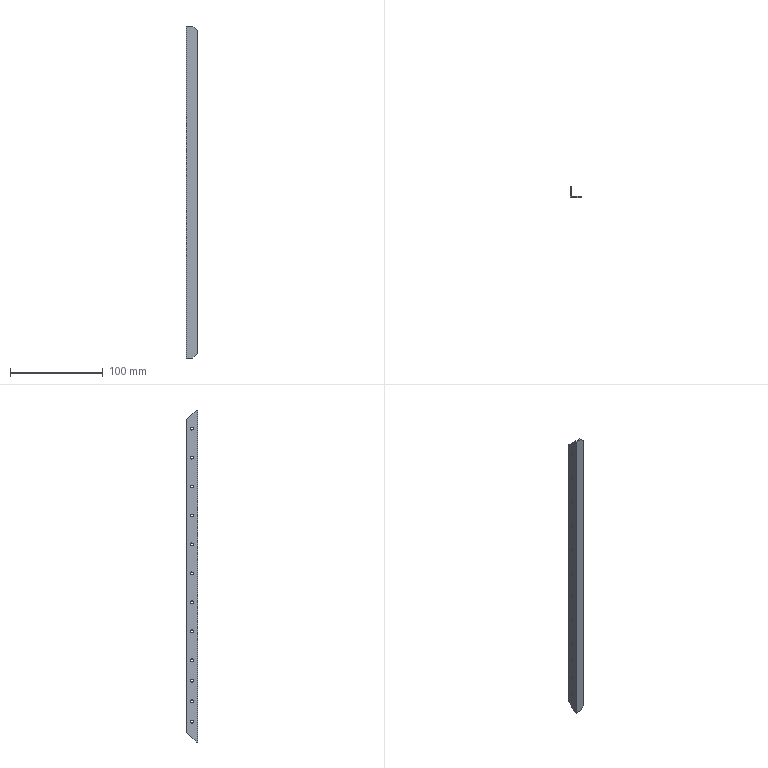Part | SolidWorks | features BaseBody 1 | 1 solid | 36 faces | box 12 x 12 x 358 mm | volume 9517 mm3 | cylinder 24 | plane 12 | commonest cylinder face diameters 3.2 x24
STEP:
#1=CARTESIAN_POINT('',(1.2,6.015,129.35));
#2=VERTEX_POINT('',#1);
#3=CARTESIAN_POINT('',(1.2,6.015,126.15));
#4=VERTEX_POINT('',#3);
#5=CARTESIAN_POINT('',(1.2,6.015,127.75));
#6=DIRECTION('',(1.,0.,0.));
#7=DIRECTION('',(0.,0.,1.));
#8=AXIS2_PLACEMENT_3D('',#5,#6,#7);
#9=CIRCLE('',#8,1.6);
#10=EDGE_CURVE('',#2,#4,#9,.T.);
#11=ORIENTED_EDGE('',*,*,#10,.T.);
#12=CARTESIAN_POINT('',(0.,6.015,126.15));
#13=VERTEX_POINT('',#12);
#14=CARTESIAN_POINT('',(1.2,6.015,126.15));
#15=DIRECTION('',(-1.,0.,0.));
#16=VECTOR('',#15,1000.);
#17=LINE('',#14,#16);
#18=EDGE_CURVE('',#4,#13,#17,.T.);
#19=ORIENTED_EDGE('',*,*,#18,.T.);
#20=CARTESIAN_POINT('',(0.,6.015,129.35));
#21=VERTEX_POINT('',#20);
#22=CARTESIAN_POINT('',(0.,6.015,127.75));
#23=DIRECTION('',(-1.,0.,0.));
#24=DIRECTION('',(0.,0.,1.));
#25=AXIS2_PLACEMENT_3D('',#22,#23,#24);
#26=CIRCLE('',#25,1.6);
#27=EDGE_CURVE('',#13,#21,#26,.T.);
#28=ORIENTED_EDGE('',*,*,#27,.T.);
#29=CARTESIAN_POINT('',(1.2,6.015,129.35));
#30=DIRECTION('',(-1.,0.,0.));
#31=VECTOR('',#30,1000.);
#32=LINE('',#29,#31);
#33=EDGE_CURVE('',#2,#21,#32,.T.);
#34=ORIENTED_EDGE('',*,*,#33,.F.);
#35=EDGE_LOOP('',(#11,#19,#28,#34));
#36=FACE_OUTER_BOUND('',#35,.T.);
#37=CARTESIAN_POINT('',(1.2,6.015,127.75));
#38=DIRECTION('',(-1.,0.,0.));
#39=DIRECTION('',(0.,0.,1.));
#40=AXIS2_PLACEMENT_3D('',#37,#38,#39);
#41=CYLINDRICAL_SURFACE('',#40,1.6);
#42=ADVANCED_FACE('',(#36),#41,.F.);
#43=CARTESIAN_POINT('',(1.2,6.015,-155.4));
#44=VERTEX_POINT('',#43);
#45=CARTESIAN_POINT('',(1.2,6.015,-158.6));
#46=VERTEX_POINT('',#45);
#47=CARTESIAN_POINT('',(1.2,6.015,-157.));
#48=DIRECTION('',(1.,0.,0.));
#49=DIRECTION('',(0.,0.,1.));
#50=AXIS2_PLACEMENT_3D('',#47,#48,#49);
#51=CIRCLE('',#50,1.6);
#52=EDGE_CURVE('',#44,#46,#51,.T.);
#53=ORIENTED_EDGE('',*,*,#52,.T.);
#54=CARTESIAN_POINT('',(0.,6.015,-158.6));
#55=VERTEX_POINT('',#54);
#56=CARTESIAN_POINT('',(1.2,6.015,-158.6));
#57=DIRECTION('',(-1.,0.,0.));
#58=VECTOR('',#57,1000.);
#59=LINE('',#56,#58);
#60=EDGE_CURVE('',#46,#55,#59,.T.);
#61=ORIENTED_EDGE('',*,*,#60,.T.);
#62=CARTESIAN_POINT('',(0.,6.015,-155.4));
#63=VERTEX_POINT('',#62);
#64=CARTESIAN_POINT('',(0.,6.015,-157.));
#65=DIRECTION('',(-1.,0.,0.));
#66=DIRECTION('',(0.,0.,1.));
#67=AXIS2_PLACEMENT_3D('',#64,#65,#66);
#68=CIRCLE('',#67,1.6);
#69=EDGE_CURVE('',#55,#63,#68,.T.);
#70=ORIENTED_EDGE('',*,*,#69,.T.);
#71=CARTESIAN_POINT('',(1.2,6.015,-155.4));
#72=DIRECTION('',(-1.,0.,0.));
#73=VECTOR('',#72,1000.);
#74=LINE('',#71,#73);
#75=EDGE_CURVE('',#44,#63,#74,.T.);
#76=ORIENTED_EDGE('',*,*,#75,.F.);
#77=EDGE_LOOP('',(#53,#61,#70,#76));
#78=FACE_OUTER_BOUND('',#77,.T.);
#79=CARTESIAN_POINT('',(1.2,6.015,-157.));
#80=DIRECTION('',(-1.,0.,0.));
#81=DIRECTION('',(0.,0.,1.));
#82=AXIS2_PLACEMENT_3D('',#79,#80,#81);
#83=CYLINDRICAL_SURFACE('',#82,1.6);
#84=ADVANCED_FACE('',(#78),#83,.F.);
#85=CARTESIAN_POINT('',(1.2,6.015,160.6));
#86=VERTEX_POINT('',#85);
#87=CARTESIAN_POINT('',(1.2,6.015,157.4));
#88=VERTEX_POINT('',#87);
#89=CARTESIAN_POINT('',(1.2,6.015,159.));
#90=DIRECTION('',(1.,0.,0.));
#91=DIRECTION('',(0.,0.,1.));
#92=AXIS2_PLACEMENT_3D('',#89,#90,#91);
#93=CIRCLE('',#92,1.6);
#94=EDGE_CURVE('',#86,#88,#93,.T.);
#95=ORIENTED_EDGE('',*,*,#94,.T.);
#96=CARTESIAN_POINT('',(0.,6.015,157.4));
#97=VERTEX_POINT('',#96);
#98=CARTESIAN_POINT('',(1.2,6.015,157.4));
#99=DIRECTION('',(-1.,0.,0.));
#100=VECTOR('',#99,1000.);
#101=LINE('',#98,#100);
#102=EDGE_CURVE('',#88,#97,#101,.T.);
#103=ORIENTED_EDGE('',*,*,#102,.T.);
#104=CARTESIAN_POINT('',(0.,6.015,160.6));
#105=VERTEX_POINT('',#104);
#106=CARTESIAN_POINT('',(0.,6.015,159.));
#107=DIRECTION('',(-1.,0.,0.));
#108=DIRECTION('',(0.,0.,1.));
#109=AXIS2_PLACEMENT_3D('',#106,#107,#108);
#110=CIRCLE('',#109,1.6);
#111=EDGE_CURVE('',#97,#105,#110,.T.);
#112=ORIENTED_EDGE('',*,*,#111,.T.);
#113=CARTESIAN_POINT('',(1.2,6.015,160.6));
#114=DIRECTION('',(-1.,0.,0.));
#115=VECTOR('',#114,1000.);
#116=LINE('',#113,#115);
#117=EDGE_CURVE('',#86,#105,#116,.T.);
#118=ORIENTED_EDGE('',*,*,#117,.F.);
#119=EDGE_LOOP('',(#95,#103,#112,#118));
#120=FACE_OUTER_BOUND('',#119,.T.);
#121=CARTESIAN_POINT('',(1.2,6.015,159.));
#122=DIRECTION('',(-1.,0.,0.));
#123=DIRECTION('',(0.,0.,1.));
#124=AXIS2_PLACEMENT_3D('',#121,#122,#123);
#125=CYLINDRICAL_SURFACE('',#124,1.6);
#126=ADVANCED_FACE('',(#120),#125,.F.);
#127=CARTESIAN_POINT('',(1.2,6.015,-133.4));
#128=VERTEX_POINT('',#127);
#129=CARTESIAN_POINT('',(1.2,6.015,-136.6));
#130=VERTEX_POINT('',#129);
#131=CARTESIAN_POINT('',(1.2,6.015,-135.));
#132=DIRECTION('',(1.,0.,0.));
#133=DIRECTION('',(0.,0.,1.));
#134=AXIS2_PLACEMENT_3D('',#131,#132,#133);
#135=CIRCLE('',#134,1.6);
#136=EDGE_CURVE('',#128,#130,#135,.T.);
#137=ORIENTED_EDGE('',*,*,#136,.T.);
#138=CARTESIAN_POINT('',(0.,6.015,-136.6));
#139=VERTEX_POINT('',#138);
#140=CARTESIAN_POINT('',(1.2,6.015,-136.6));
#141=DIRECTION('',(-1.,0.,0.));
#142=VECTOR('',#141,1000.);
#143=LINE('',#140,#142);
#144=EDGE_CURVE('',#130,#139,#143,.T.);
#145=ORIENTED_EDGE('',*,*,#144,.T.);
#146=CARTESIAN_POINT('',(0.,6.015,-133.4));
#147=VERTEX_POINT('',#146);
#148=CARTESIAN_POINT('',(0.,6.015,-135.));
#149=DIRECTION('',(-1.,0.,0.));
#150=DIRECTION('',(0.,0.,1.));
#151=AXIS2_PLACEMENT_3D('',#148,#149,#150);
#152=CIRCLE('',#151,1.6);
#153=EDGE_CURVE('',#139,#147,#152,.T.);
#154=ORIENTED_EDGE('',*,*,#153,.T.);
#155=CARTESIAN_POINT('',(1.2,6.015,-133.4));
#156=DIRECTION('',(-1.,0.,0.));
#157=VECTOR('',#156,1000.);
#158=LINE('',#155,#157);
#159=EDGE_CURVE('',#128,#147,#158,.T.);
#160=ORIENTED_EDGE('',*,*,#159,.F.);
#161=EDGE_LOOP('',(#137,#145,#154,#160));
#162=FACE_OUTER_BOUND('',#161,.T.);
#163=CARTESIAN_POINT('',(1.2,6.015,-135.));
#164=DIRECTION('',(-1.,0.,0.));
#165=DIRECTION('',(0.,0.,1.));
#166=AXIS2_PLACEMENT_3D('',#163,#164,#165);
#167=CYLINDRICAL_SURFACE('',#166,1.6);
#168=ADVANCED_FACE('',(#162),#167,.F.);
#169=CARTESIAN_POINT('',(1.2,6.015,-111.4));
#170=VERTEX_POINT('',#169);
#171=CARTESIAN_POINT('',(1.2,6.015,-114.6));
#172=VERTEX_POINT('',#171);
#173=CARTESIAN_POINT('',(1.2,6.015,-113.));
#174=DIRECTION('',(1.,0.,0.));
#175=DIRECTION('',(0.,0.,1.));
#176=AXIS2_PLACEMENT_3D('',#173,#174,#175);
#177=CIRCLE('',#176,1.6);
#178=EDGE_CURVE('',#170,#172,#177,.T.);
#179=ORIENTED_EDGE('',*,*,#178,.T.);
#180=CARTESIAN_POINT('',(0.,6.015,-114.6));
#181=VERTEX_POINT('',#180);
#182=CARTESIAN_POINT('',(1.2,6.015,-114.6));
#183=DIRECTION('',(-1.,0.,0.));
#184=VECTOR('',#183,1000.);
#185=LINE('',#182,#184);
#186=EDGE_CURVE('',#172,#181,#185,.T.);
#187=ORIENTED_EDGE('',*,*,#186,.T.);
#188=CARTESIAN_POINT('',(0.,6.015,-111.4));
#189=VERTEX_POINT('',#188);
#190=CARTESIAN_POINT('',(0.,6.015,-113.));
#191=DIRECTION('',(-1.,0.,0.));
#192=DIRECTION('',(0.,0.,1.));
#193=AXIS2_PLACEMENT_3D('',#190,#191,#192);
#194=CIRCLE('',#193,1.6);
#195=EDGE_CURVE('',#181,#189,#194,.T.);
#196=ORIENTED_EDGE('',*,*,#195,.T.);
#197=CARTESIAN_POINT('',(1.2,6.015,-111.4));
#198=DIRECTION('',(-1.,0.,0.));
#199=VECTOR('',#198,1000.);
#200=LINE('',#197,#199);
#201=EDGE_CURVE('',#170,#189,#200,.T.);
#202=ORIENTED_EDGE('',*,*,#201,.F.);
#203=EDGE_LOOP('',(#179,#187,#196,#202));
#204=FACE_OUTER_BOUND('',#203,.T.);
#205=CARTESIAN_POINT('',(1.2,6.015,-113.));
#206=DIRECTION('',(-1.,0.,0.));
#207=DIRECTION('',(0.,0.,1.));
#208=AXIS2_PLACEMENT_3D('',#205,#206,#207);
#209=CYLINDRICAL_SURFACE('',#208,1.6);
#210=ADVANCED_FACE('',(#204),#209,.F.);
#211=CARTESIAN_POINT('',(1.2,6.015,-89.4));
#212=VERTEX_POINT('',#211);
#213=CARTESIAN_POINT('',(1.2,6.015,-92.6));
#214=VERTEX_POINT('',#213);
#215=CARTESIAN_POINT('',(1.2,6.015,-91.));
#216=DIRECTION('',(1.,0.,0.));
#217=DIRECTION('',(0.,0.,1.));
#218=AXIS2_PLACEMENT_3D('',#215,#216,#217);
#219=CIRCLE('',#218,1.6);
#220=EDGE_CURVE('',#212,#214,#219,.T.);
#221=ORIENTED_EDGE('',*,*,#220,.T.);
#222=CARTESIAN_POINT('',(0.,6.015,-92.6));
#223=VERTEX_POINT('',#222);
#224=CARTESIAN_POINT('',(1.2,6.015,-92.6));
#225=DIRECTION('',(-1.,0.,0.));
#226=VECTOR('',#225,1000.);
#227=LINE('',#224,#226);
#228=EDGE_CURVE('',#214,#223,#227,.T.);
#229=ORIENTED_EDGE('',*,*,#228,.T.);
#230=CARTESIAN_POINT('',(0.,6.015,-89.4));
#231=VERTEX_POINT('',#230);
#232=CARTESIAN_POINT('',(0.,6.015,-91.));
#233=DIRECTION('',(-1.,0.,0.));
#234=DIRECTION('',(0.,0.,1.));
#235=AXIS2_PLACEMENT_3D('',#232,#233,#234);
#236=CIRCLE('',#235,1.6);
#237=EDGE_CURVE('',#223,#231,#236,.T.);
#238=ORIENTED_EDGE('',*,*,#237,.T.);
#239=CARTESIAN_POINT('',(1.2,6.015,-89.4));
#240=DIRECTION('',(-1.,0.,0.));
#241=VECTOR('',#240,1000.);
#242=LINE('',#239,#241);
#243=EDGE_CURVE('',#212,#231,#242,.T.);
#244=ORIENTED_EDGE('',*,*,#243,.F.);
#245=EDGE_LOOP('',(#221,#229,#238,#244));
#246=FACE_OUTER_BOUND('',#245,.T.);
#247=CARTESIAN_POINT('',(1.2,6.015,-91.));
#248=DIRECTION('',(-1.,0.,0.));
#249=DIRECTION('',(0.,0.,1.));
#250=AXIS2_PLACEMENT_3D('',#247,#248,#249);
#251=CYLINDRICAL_SURFACE('',#250,1.6);
#252=ADVANCED_FACE('',(#246),#251,.F.);
#253=CARTESIAN_POINT('',(1.2,6.015,-58.15));
#254=VERTEX_POINT('',#253);
#255=CARTESIAN_POINT('',(1.2,6.015,-61.35));
#256=VERTEX_POINT('',#255);
#257=CARTESIAN_POINT('',(1.2,6.015,-59.75));
#258=DIRECTION('',(1.,0.,0.));
#259=DIRECTION('',(0.,0.,1.));
#260=AXIS2_PLACEMENT_3D('',#257,#258,#259);
#261=CIRCLE('',#260,1.6);
#262=EDGE_CURVE('',#254,#256,#261,.T.);
#263=ORIENTED_EDGE('',*,*,#262,.T.);
#264=CARTESIAN_POINT('',(0.,6.015,-61.35));
#265=VERTEX_POINT('',#264);
#266=CARTESIAN_POINT('',(1.2,6.015,-61.35));
#267=DIRECTION('',(-1.,0.,0.));
#268=VECTOR('',#267,1000.);
#269=LINE('',#266,#268);
#270=EDGE_CURVE('',#256,#265,#269,.T.);
#271=ORIENTED_EDGE('',*,*,#270,.T.);
#272=CARTESIAN_POINT('',(0.,6.015,-58.15));
#273=VERTEX_POINT('',#272);
#274=CARTESIAN_POINT('',(0.,6.015,-59.75));
#275=DIRECTION('',(-1.,0.,0.));
#276=DIRECTION('',(0.,0.,1.));
#277=AXIS2_PLACEMENT_3D('',#274,#275,#276);
#278=CIRCLE('',#277,1.6);
#279=EDGE_CURVE('',#265,#273,#278,.T.);
#280=ORIENTED_EDGE('',*,*,#279,.T.);
#281=CARTESIAN_POINT('',(1.2,6.015,-58.15));
#282=DIRECTION('',(-1.,0.,0.));
#283=VECTOR('',#282,1000.);
#284=LINE('',#281,#283);
#285=EDGE_CURVE('',#254,#273,#284,.T.);
#286=ORIENTED_EDGE('',*,*,#285,.F.);
#287=EDGE_LOOP('',(#263,#271,#280,#286));
#288=FACE_OUTER_BOUND('',#287,.T.);
#289=CARTESIAN_POINT('',(1.2,6.015,-59.75));
#290=DIRECTION('',(-1.,0.,0.));
#291=DIRECTION('',(0.,0.,1.));
#292=AXIS2_PLACEMENT_3D('',#289,#290,#291);
#293=CYLINDRICAL_SURFACE('',#292,1.6);
#294=ADVANCED_FACE('',(#288),#293,.F.);
#295=CARTESIAN_POINT('',(1.2,6.015,-26.9));
#296=VERTEX_POINT('',#295);
#297=CARTESIAN_POINT('',(1.2,6.015,-30.1));
#298=VERTEX_POINT('',#297);
#299=CARTESIAN_POINT('',(1.2,6.015,-28.5));
#300=DIRECTION('',(1.,0.,0.));
#301=DIRECTION('',(0.,0.,1.));
#302=AXIS2_PLACEMENT_3D('',#299,#300,#301);
#303=CIRCLE('',#302,1.6);
#304=EDGE_CURVE('',#296,#298,#303,.T.);
#305=ORIENTED_EDGE('',*,*,#304,.T.);
#306=CARTESIAN_POINT('',(0.,6.015,-30.1));
#307=VERTEX_POINT('',#306);
#308=CARTESIAN_POINT('',(1.2,6.015,-30.1));
#309=DIRECTION('',(-1.,0.,0.));
#310=VECTOR('',#309,1000.);
#311=LINE('',#308,#310);
#312=EDGE_CURVE('',#298,#307,#311,.T.);
#313=ORIENTED_EDGE('',*,*,#312,.T.);
#314=CARTESIAN_POINT('',(0.,6.015,-26.9));
#315=VERTEX_POINT('',#314);
#316=CARTESIAN_POINT('',(0.,6.015,-28.5));
#317=DIRECTION('',(-1.,0.,0.));
#318=DIRECTION('',(0.,0.,1.));
#319=AXIS2_PLACEMENT_3D('',#316,#317,#318);
#320=CIRCLE('',#319,1.6);
#321=EDGE_CURVE('',#307,#315,#320,.T.);
#322=ORIENTED_EDGE('',*,*,#321,.T.);
#323=CARTESIAN_POINT('',(1.2,6.015,-26.9));
#324=DIRECTION('',(-1.,0.,0.));
#325=VECTOR('',#324,1000.);
#326=LINE('',#323,#325);
#327=EDGE_CURVE('',#296,#315,#326,.T.);
#328=ORIENTED_EDGE('',*,*,#327,.F.);
#329=EDGE_LOOP('',(#305,#313,#322,#328));
#330=FACE_OUTER_BOUND('',#329,.T.);
#331=CARTESIAN_POINT('',(1.2,6.015,-28.5));
#332=DIRECTION('',(-1.,0.,0.));
#333=DIRECTION('',(0.,0.,1.));
#334=AXIS2_PLACEMENT_3D('',#331,#332,#333);
#335=CYLINDRICAL_SURFACE('',#334,1.6);
#336=ADVANCED_FACE('',(#330),#335,.F.);
#337=CARTESIAN_POINT('',(1.2,6.015,4.35));
#338=VERTEX_POINT('',#337);
#339=CARTESIAN_POINT('',(1.2,6.015,1.15));
#340=VERTEX_POINT('',#339);
#341=CARTESIAN_POINT('',(1.2,6.015,2.75));
#342=DIRECTION('',(1.,0.,0.));
#343=DIRECTION('',(0.,0.,1.));
#344=AXIS2_PLACEMENT_3D('',#341,#342,#343);
#345=CIRCLE('',#344,1.6);
#346=EDGE_CURVE('',#338,#340,#345,.T.);
#347=ORIENTED_EDGE('',*,*,#346,.T.);
#348=CARTESIAN_POINT('',(0.,6.015,1.15));
#349=VERTEX_POINT('',#348);
#350=CARTESIAN_POINT('',(1.2,6.015,1.15));
#351=DIRECTION('',(-1.,0.,0.));
#352=VECTOR('',#351,1000.);
#353=LINE('',#350,#352);
#354=EDGE_CURVE('',#340,#349,#353,.T.);
#355=ORIENTED_EDGE('',*,*,#354,.T.);
#356=CARTESIAN_POINT('',(0.,6.015,4.35));
#357=VERTEX_POINT('',#356);
#358=CARTESIAN_POINT('',(0.,6.015,2.75));
#359=DIRECTION('',(-1.,0.,0.));
#360=DIRECTION('',(0.,0.,1.));
#361=AXIS2_PLACEMENT_3D('',#358,#359,#360);
#362=CIRCLE('',#361,1.6);
#363=EDGE_CURVE('',#349,#357,#362,.T.);
#364=ORIENTED_EDGE('',*,*,#363,.T.);
#365=CARTESIAN_POINT('',(1.2,6.015,4.35));
#366=DIRECTION('',(-1.,0.,0.));
#367=VECTOR('',#366,1000.);
#368=LINE('',#365,#367);
#369=EDGE_CURVE('',#338,#357,#368,.T.);
#370=ORIENTED_EDGE('',*,*,#369,.F.);
#371=EDGE_LOOP('',(#347,#355,#364,#370));
#372=FACE_OUTER_BOUND('',#371,.T.);
#373=CARTESIAN_POINT('',(1.2,6.015,2.75));
#374=DIRECTION('',(-1.,0.,0.));
#375=DIRECTION('',(0.,0.,1.));
#376=AXIS2_PLACEMENT_3D('',#373,#374,#375);
#377=CYLINDRICAL_SURFACE('',#376,1.6);
#378=ADVANCED_FACE('',(#372),#377,.F.);
#379=CARTESIAN_POINT('',(1.2,6.015,35.6));
#380=VERTEX_POINT('',#379);
#381=CARTESIAN_POINT('',(1.2,6.015,32.4));
#382=VERTEX_POINT('',#381);
#383=CARTESIAN_POINT('',(1.2,6.015,34.));
#384=DIRECTION('',(1.,0.,0.));
#385=DIRECTION('',(0.,0.,1.));
#386=AXIS2_PLACEMENT_3D('',#383,#384,#385);
#387=CIRCLE('',#386,1.6);
#388=EDGE_CURVE('',#380,#382,#387,.T.);
#389=ORIENTED_EDGE('',*,*,#388,.T.);
#390=CARTESIAN_POINT('',(0.,6.015,32.4));
#391=VERTEX_POINT('',#390);
#392=CARTESIAN_POINT('',(1.2,6.015,32.4));
#393=DIRECTION('',(-1.,0.,0.));
#394=VECTOR('',#393,1000.);
#395=LINE('',#392,#394);
#396=EDGE_CURVE('',#382,#391,#395,.T.);
#397=ORIENTED_EDGE('',*,*,#396,.T.);
#398=CARTESIAN_POINT('',(0.,6.015,35.6));
#399=VERTEX_POINT('',#398);
#400=CARTESIAN_POINT('',(0.,6.015,34.));
#401=DIRECTION('',(-1.,0.,0.));
#402=DIRECTION('',(0.,0.,1.));
#403=AXIS2_PLACEMENT_3D('',#400,#401,#402);
#404=CIRCLE('',#403,1.6);
#405=EDGE_CURVE('',#391,#399,#404,.T.);
#406=ORIENTED_EDGE('',*,*,#405,.T.);
#407=CARTESIAN_POINT('',(1.2,6.015,35.6));
#408=DIRECTION('',(-1.,0.,0.));
#409=VECTOR('',#408,1000.);
#410=LINE('',#407,#409);
#411=EDGE_CURVE('',#380,#399,#410,.T.);
#412=ORIENTED_EDGE('',*,*,#411,.F.);
#413=EDGE_LOOP('',(#389,#397,#406,#412));
#414=FACE_OUTER_BOUND('',#413,.T.);
#415=CARTESIAN_POINT('',(1.2,6.015,34.));
#416=DIRECTION('',(-1.,0.,0.));
#417=DIRECTION('',(0.,0.,1.));
#418=AXIS2_PLACEMENT_3D('',#415,#416,#417);
#419=CYLINDRICAL_SURFACE('',#418,1.6);
#420=ADVANCED_FACE('',(#414),#419,.F.);
#421=CARTESIAN_POINT('',(1.2,6.015,66.85));
#422=VERTEX_POINT('',#421);
#423=CARTESIAN_POINT('',(1.2,6.015,63.65));
#424=VERTEX_POINT('',#423);
#425=CARTESIAN_POINT('',(1.2,6.015,65.25));
#426=DIRECTION('',(1.,0.,0.));
#427=DIRECTION('',(0.,0.,1.));
#428=AXIS2_PLACEMENT_3D('',#425,#426,#427);
#429=CIRCLE('',#428,1.6);
#430=EDGE_CURVE('',#422,#424,#429,.T.);
#431=ORIENTED_EDGE('',*,*,#430,.T.);
#432=CARTESIAN_POINT('',(0.,6.015,63.65));
#433=VERTEX_POINT('',#432);
#434=CARTESIAN_POINT('',(1.2,6.015,63.65));
#435=DIRECTION('',(-1.,0.,0.));
#436=VECTOR('',#435,1000.);
#437=LINE('',#434,#436);
#438=EDGE_CURVE('',#424,#433,#437,.T.);
#439=ORIENTED_EDGE('',*,*,#438,.T.);
#440=CARTESIAN_POINT('',(0.,6.015,66.85));
#441=VERTEX_POINT('',#440);
#442=CARTESIAN_POINT('',(0.,6.015,65.25));
#443=DIRECTION('',(-1.,0.,0.));
#444=DIRECTION('',(0.,0.,1.));
#445=AXIS2_PLACEMENT_3D('',#442,#443,#444);
#446=CIRCLE('',#445,1.6);
#447=EDGE_CURVE('',#433,#441,#446,.T.);
#448=ORIENTED_EDGE('',*,*,#447,.T.);
#449=CARTESIAN_POINT('',(1.2,6.015,66.85));
#450=DIRECTION('',(-1.,0.,0.));
#451=VECTOR('',#450,1000.);
#452=LINE('',#449,#451);
#453=EDGE_CURVE('',#422,#441,#452,.T.);
#454=ORIENTED_EDGE('',*,*,#453,.F.);
#455=EDGE_LOOP('',(#431,#439,#448,#454));
#456=FACE_OUTER_BOUND('',#455,.T.);
#457=CARTESIAN_POINT('',(1.2,6.015,65.25));
#458=DIRECTION('',(-1.,0.,0.));
#459=DIRECTION('',(0.,0.,1.));
#460=AXIS2_PLACEMENT_3D('',#457,#458,#459);
#461=CYLINDRICAL_SURFACE('',#460,1.6);
#462=ADVANCED_FACE('',(#456),#461,.F.);
#463=CARTESIAN_POINT('',(1.2,6.015,98.1));
#464=VERTEX_POINT('',#463);
#465=CARTESIAN_POINT('',(1.2,6.015,94.9));
#466=VERTEX_POINT('',#465);
#467=CARTESIAN_POINT('',(1.2,6.015,96.5));
#468=DIRECTION('',(1.,0.,0.));
#469=DIRECTION('',(0.,0.,1.));
#470=AXIS2_PLACEMENT_3D('',#467,#468,#469);
#471=CIRCLE('',#470,1.6);
#472=EDGE_CURVE('',#464,#466,#471,.T.);
#473=ORIENTED_EDGE('',*,*,#472,.T.);
#474=CARTESIAN_POINT('',(0.,6.015,94.9));
#475=VERTEX_POINT('',#474);
#476=CARTESIAN_POINT('',(1.2,6.015,94.9));
#477=DIRECTION('',(-1.,0.,0.));
#478=VECTOR('',#477,1000.);
#479=LINE('',#476,#478);
#480=EDGE_CURVE('',#466,#475,#479,.T.);
#481=ORIENTED_EDGE('',*,*,#480,.T.);
#482=CARTESIAN_POINT('',(0.,6.015,98.1));
#483=VERTEX_POINT('',#482);
#484=CARTESIAN_POINT('',(0.,6.015,96.5));
#485=DIRECTION('',(-1.,0.,0.));
#486=DIRECTION('',(0.,0.,1.));
#487=AXIS2_PLACEMENT_3D('',#484,#485,#486);
#488=CIRCLE('',#487,1.6);
#489=EDGE_CURVE('',#475,#483,#488,.T.);
#490=ORIENTED_EDGE('',*,*,#489,.T.);
#491=CARTESIAN_POINT('',(1.2,6.015,98.1));
#492=DIRECTION('',(-1.,0.,0.));
#493=VECTOR('',#492,1000.);
#494=LINE('',#491,#493);
#495=EDGE_CURVE('',#464,#483,#494,.T.);
#496=ORIENTED_EDGE('',*,*,#495,.F.);
#497=EDGE_LOOP('',(#473,#481,#490,#496));
#498=FACE_OUTER_BOUND('',#497,.T.);
#499=CARTESIAN_POINT('',(1.2,6.015,96.5));
#500=DIRECTION('',(-1.,0.,0.));
#501=DIRECTION('',(0.,0.,1.));
#502=AXIS2_PLACEMENT_3D('',#499,#500,#501);
#503=CYLINDRICAL_SURFACE('',#502,1.6);
#504=ADVANCED_FACE('',(#498),#503,.F.);
#505=ORIENTED_EDGE('',*,*,#18,.F.);
#506=CARTESIAN_POINT('',(1.2,6.015,127.75));
#507=DIRECTION('',(1.,0.,0.));
#508=DIRECTION('',(0.,0.,1.));
#509=AXIS2_PLACEMENT_3D('',#506,#507,#508);
#510=CIRCLE('',#509,1.6);
#511=EDGE_CURVE('',#4,#2,#510,.T.);
#512=ORIENTED_EDGE('',*,*,#511,.T.);
#513=ORIENTED_EDGE('',*,*,#33,.T.);
#514=CARTESIAN_POINT('',(0.,6.015,127.75));
#515=DIRECTION('',(-1.,0.,0.));
#516=DIRECTION('',(0.,0.,1.));
#517=AXIS2_PLACEMENT_3D('',#514,#515,#516);
#518=CIRCLE('',#517,1.6);
#519=EDGE_CURVE('',#21,#13,#518,.T.);
#520=ORIENTED_EDGE('',*,*,#519,.T.);
#521=EDGE_LOOP('',(#505,#512,#513,#520));
#522=FACE_OUTER_BOUND('',#521,.T.);
#523=CARTESIAN_POINT('',(1.2,6.015,127.75));
#524=DIRECTION('',(-1.,0.,0.));
#525=DIRECTION('',(0.,0.,1.));
#526=AXIS2_PLACEMENT_3D('',#523,#524,#525);
#527=CYLINDRICAL_SURFACE('',#526,1.6);
#528=ADVANCED_FACE('',(#522),#527,.F.);
#529=CARTESIAN_POINT('',(0.,6.015,-157.));
#530=DIRECTION('',(-1.,0.,0.));
#531=DIRECTION('',(0.,0.,1.));
#532=AXIS2_PLACEMENT_3D('',#529,#530,#531);
#533=CIRCLE('',#532,1.6);
#534=EDGE_CURVE('',#63,#55,#533,.T.);
#535=ORIENTED_EDGE('',*,*,#534,.F.);
#536=ORIENTED_EDGE('',*,*,#69,.F.);
#537=EDGE_LOOP('',(#535,#536));
#538=FACE_BOUND('',#537,.T.);
#539=CARTESIAN_POINT('',(0.,6.015,159.));
#540=DIRECTION('',(-1.,0.,0.));
#541=DIRECTION('',(0.,0.,1.));
#542=AXIS2_PLACEMENT_3D('',#539,#540,#541);
#543=CIRCLE('',#542,1.6);
#544=EDGE_CURVE('',#105,#97,#543,.T.);
#545=ORIENTED_EDGE('',*,*,#544,.F.);
#546=ORIENTED_EDGE('',*,*,#111,.F.);
#547=EDGE_LOOP('',(#545,#546));
#548=FACE_BOUND('',#547,.T.);
#549=CARTESIAN_POINT('',(0.,6.015,-135.));
#550=DIRECTION('',(-1.,0.,0.));
#551=DIRECTION('',(0.,0.,1.));
#552=AXIS2_PLACEMENT_3D('',#549,#550,#551);
#553=CIRCLE('',#552,1.6);
#554=EDGE_CURVE('',#147,#139,#553,.T.);
#555=ORIENTED_EDGE('',*,*,#554,.F.);
#556=ORIENTED_EDGE('',*,*,#153,.F.);
#557=EDGE_LOOP('',(#555,#556));
#558=FACE_BOUND('',#557,.T.);
#559=CARTESIAN_POINT('',(0.,6.015,-113.));
#560=DIRECTION('',(-1.,0.,0.));
#561=DIRECTION('',(0.,0.,1.));
#562=AXIS2_PLACEMENT_3D('',#559,#560,#561);
#563=CIRCLE('',#562,1.6);
#564=EDGE_CURVE('',#189,#181,#563,.T.);
#565=ORIENTED_EDGE('',*,*,#564,.F.);
#566=ORIENTED_EDGE('',*,*,#195,.F.);
#567=EDGE_LOOP('',(#565,#566));
#568=FACE_BOUND('',#567,.T.);
#569=CARTESIAN_POINT('',(0.,6.015,-91.));
#570=DIRECTION('',(-1.,0.,0.));
#571=DIRECTION('',(0.,0.,1.));
#572=AXIS2_PLACEMENT_3D('',#569,#570,#571);
#573=CIRCLE('',#572,1.6);
#574=EDGE_CURVE('',#231,#223,#573,.T.);
#575=ORIENTED_EDGE('',*,*,#574,.F.);
#576=ORIENTED_EDGE('',*,*,#237,.F.);
#577=EDGE_LOOP('',(#575,#576));
#578=FACE_BOUND('',#577,.T.);
#579=CARTESIAN_POINT('',(0.,6.015,-59.75));
#580=DIRECTION('',(-1.,0.,0.));
#581=DIRECTION('',(0.,0.,1.));
#582=AXIS2_PLACEMENT_3D('',#579,#580,#581);
#583=CIRCLE('',#582,1.6);
#584=EDGE_CURVE('',#273,#265,#583,.T.);
#585=ORIENTED_EDGE('',*,*,#584,.F.);
#586=ORIENTED_EDGE('',*,*,#279,.F.);
#587=EDGE_LOOP('',(#585,#586));
#588=FACE_BOUND('',#587,.T.);
#589=CARTESIAN_POINT('',(0.,6.015,-28.5));
#590=DIRECTION('',(-1.,0.,0.));
#591=DIRECTION('',(0.,0.,1.));
#592=AXIS2_PLACEMENT_3D('',#589,#590,#591);
#593=CIRCLE('',#592,1.6);
#594=EDGE_CURVE('',#315,#307,#593,.T.);
#595=ORIENTED_EDGE('',*,*,#594,.F.);
#596=ORIENTED_EDGE('',*,*,#321,.F.);
#597=EDGE_LOOP('',(#595,#596));
#598=FACE_BOUND('',#597,.T.);
#599=CARTESIAN_POINT('',(0.,6.015,2.75));
#600=DIRECTION('',(-1.,0.,0.));
#601=DIRECTION('',(0.,0.,1.));
#602=AXIS2_PLACEMENT_3D('',#599,#600,#601);
#603=CIRCLE('',#602,1.6);
#604=EDGE_CURVE('',#357,#349,#603,.T.);
#605=ORIENTED_EDGE('',*,*,#604,.F.);
#606=ORIENTED_EDGE('',*,*,#363,.F.);
#607=EDGE_LOOP('',(#605,#606));
#608=FACE_BOUND('',#607,.T.);
#609=CARTESIAN_POINT('',(0.,6.015,34.));
#610=DIRECTION('',(-1.,0.,0.));
#611=DIRECTION('',(0.,0.,1.));
#612=AXIS2_PLACEMENT_3D('',#609,#610,#611);
#613=CIRCLE('',#612,1.6);
#614=EDGE_CURVE('',#399,#391,#613,.T.);
#615=ORIENTED_EDGE('',*,*,#614,.F.);
#616=ORIENTED_EDGE('',*,*,#405,.F.);
#617=EDGE_LOOP('',(#615,#616));
#618=FACE_BOUND('',#617,.T.);
#619=CARTESIAN_POINT('',(0.,6.015,65.25));
#620=DIRECTION('',(-1.,0.,0.));
#621=DIRECTION('',(0.,0.,1.));
#622=AXIS2_PLACEMENT_3D('',#619,#620,#621);
#623=CIRCLE('',#622,1.6);
#624=EDGE_CURVE('',#441,#433,#623,.T.);
#625=ORIENTED_EDGE('',*,*,#624,.F.);
#626=ORIENTED_EDGE('',*,*,#447,.F.);
#627=EDGE_LOOP('',(#625,#626));
#628=FACE_BOUND('',#627,.T.);
#629=CARTESIAN_POINT('',(0.,6.015,96.5));
#630=DIRECTION('',(-1.,0.,0.));
#631=DIRECTION('',(0.,0.,1.));
#632=AXIS2_PLACEMENT_3D('',#629,#630,#631);
#633=CIRCLE('',#632,1.6);
#634=EDGE_CURVE('',#483,#475,#633,.T.);
#635=ORIENTED_EDGE('',*,*,#634,.F.);
#636=ORIENTED_EDGE('',*,*,#489,.F.);
#637=EDGE_LOOP('',(#635,#636));
#638=FACE_BOUND('',#637,.T.);
#639=ORIENTED_EDGE('',*,*,#519,.F.);
#640=ORIENTED_EDGE('',*,*,#27,.F.);
#641=EDGE_LOOP('',(#639,#640));
#642=FACE_BOUND('',#641,.T.);
#643=CARTESIAN_POINT('',(0.,1.5,-179.));
#644=VERTEX_POINT('',#643);
#645=CARTESIAN_POINT('',(0.,12.,-168.5));
#646=VERTEX_POINT('',#645);
#647=CARTESIAN_POINT('',(0.,1.5,-179.));
#648=DIRECTION('',(0.,0.7071,0.7071));
#649=VECTOR('',#648,1000.);
#650=LINE('',#647,#649);
#651=EDGE_CURVE('',#644,#646,#650,.T.);
#652=ORIENTED_EDGE('',*,*,#651,.F.);
#653=CARTESIAN_POINT('',(0.,0.,-179.));
#654=VERTEX_POINT('',#653);
#655=CARTESIAN_POINT('',(0.,0.75,-179.));
#656=DIRECTION('',(0.,-1.,0.));
#657=VECTOR('',#656,1000.);
#658=LINE('',#655,#657);
#659=EDGE_CURVE('',#644,#654,#658,.T.);
#660=ORIENTED_EDGE('',*,*,#659,.T.);
#661=CARTESIAN_POINT('',(0.,0.,179.));
#662=VERTEX_POINT('',#661);
#663=CARTESIAN_POINT('',(0.,0.,0.));
#664=DIRECTION('',(0.,0.,-1.));
#665=VECTOR('',#664,1000.);
#666=LINE('',#663,#665);
#667=EDGE_CURVE('',#662,#654,#666,.T.);
#668=ORIENTED_EDGE('',*,*,#667,.F.);
#669=CARTESIAN_POINT('',(0.,1.5,179.));
#670=VERTEX_POINT('',#669);
#671=CARTESIAN_POINT('',(0.,0.75,179.));
#672=DIRECTION('',(0.,-1.,0.));
#673=VECTOR('',#672,1000.);
#674=LINE('',#671,#673);
#675=EDGE_CURVE('',#670,#662,#674,.T.);
#676=ORIENTED_EDGE('',*,*,#675,.F.);
#677=CARTESIAN_POINT('',(0.,12.,168.5));
#678=VERTEX_POINT('',#677);
#679=CARTESIAN_POINT('',(0.,1.5,179.));
#680=DIRECTION('',(0.,-0.7071,0.7071));
#681=VECTOR('',#680,1000.);
#682=LINE('',#679,#681);
#683=EDGE_CURVE('',#678,#670,#682,.T.);
#684=ORIENTED_EDGE('',*,*,#683,.F.);
#685=CARTESIAN_POINT('',(0.,12.,0.));
#686=DIRECTION('',(0.,0.,1.));
#687=VECTOR('',#686,1000.);
#688=LINE('',#685,#687);
#689=EDGE_CURVE('',#646,#678,#688,.T.);
#690=ORIENTED_EDGE('',*,*,#689,.F.);
#691=EDGE_LOOP('',(#652,#660,#668,#676,#684,#690));
#692=FACE_OUTER_BOUND('',#691,.T.);
#693=CARTESIAN_POINT('',(0.,12.,-179.));
#694=DIRECTION('',(1.,0.,0.));
#695=DIRECTION('',(0.,0.,1.));
#696=AXIS2_PLACEMENT_3D('',#693,#694,#695);
#697=PLANE('',#696);
#698=ADVANCED_FACE('',(#538,#548,#558,#568,#578,#588,#598,#608,#618,#628,#638,#642,#692),#697,.F.);
#699=ORIENTED_EDGE('',*,*,#52,.F.);
#700=CARTESIAN_POINT('',(1.2,6.015,-157.));
#701=DIRECTION('',(1.,0.,0.));
#702=DIRECTION('',(0.,0.,1.));
#703=AXIS2_PLACEMENT_3D('',#700,#701,#702);
#704=CIRCLE('',#703,1.6);
#705=EDGE_CURVE('',#46,#44,#704,.T.);
#706=ORIENTED_EDGE('',*,*,#705,.F.);
#707=EDGE_LOOP('',(#699,#706));
#708=FACE_BOUND('',#707,.T.);
#709=ORIENTED_EDGE('',*,*,#94,.F.);
#710=CARTESIAN_POINT('',(1.2,6.015,159.));
#711=DIRECTION('',(1.,0.,0.));
#712=DIRECTION('',(0.,0.,1.));
#713=AXIS2_PLACEMENT_3D('',#710,#711,#712);
#714=CIRCLE('',#713,1.6);
#715=EDGE_CURVE('',#88,#86,#714,.T.);
#716=ORIENTED_EDGE('',*,*,#715,.F.);
#717=EDGE_LOOP('',(#709,#716));
#718=FACE_BOUND('',#717,.T.);
#719=ORIENTED_EDGE('',*,*,#136,.F.);
#720=CARTESIAN_POINT('',(1.2,6.015,-135.));
#721=DIRECTION('',(1.,0.,0.));
#722=DIRECTION('',(0.,0.,1.));
#723=AXIS2_PLACEMENT_3D('',#720,#721,#722);
#724=CIRCLE('',#723,1.6);
#725=EDGE_CURVE('',#130,#128,#724,.T.);
#726=ORIENTED_EDGE('',*,*,#725,.F.);
#727=EDGE_LOOP('',(#719,#726));
#728=FACE_BOUND('',#727,.T.);
#729=ORIENTED_EDGE('',*,*,#178,.F.);
#730=CARTESIAN_POINT('',(1.2,6.015,-113.));
#731=DIRECTION('',(1.,0.,0.));
#732=DIRECTION('',(0.,0.,1.));
#733=AXIS2_PLACEMENT_3D('',#730,#731,#732);
#734=CIRCLE('',#733,1.6);
#735=EDGE_CURVE('',#172,#170,#734,.T.);
#736=ORIENTED_EDGE('',*,*,#735,.F.);
#737=EDGE_LOOP('',(#729,#736));
#738=FACE_BOUND('',#737,.T.);
#739=ORIENTED_EDGE('',*,*,#220,.F.);
#740=CARTESIAN_POINT('',(1.2,6.015,-91.));
#741=DIRECTION('',(1.,0.,0.));
#742=DIRECTION('',(0.,0.,1.));
#743=AXIS2_PLACEMENT_3D('',#740,#741,#742);
#744=CIRCLE('',#743,1.6);
#745=EDGE_CURVE('',#214,#212,#744,.T.);
#746=ORIENTED_EDGE('',*,*,#745,.F.);
#747=EDGE_LOOP('',(#739,#746));
#748=FACE_BOUND('',#747,.T.);
#749=ORIENTED_EDGE('',*,*,#262,.F.);
#750=CARTESIAN_POINT('',(1.2,6.015,-59.75));
#751=DIRECTION('',(1.,0.,0.));
#752=DIRECTION('',(0.,0.,1.));
#753=AXIS2_PLACEMENT_3D('',#750,#751,#752);
#754=CIRCLE('',#753,1.6);
#755=EDGE_CURVE('',#256,#254,#754,.T.);
#756=ORIENTED_EDGE('',*,*,#755,.F.);
#757=EDGE_LOOP('',(#749,#756));
#758=FACE_BOUND('',#757,.T.);
#759=ORIENTED_EDGE('',*,*,#304,.F.);
#760=CARTESIAN_POINT('',(1.2,6.015,-28.5));
#761=DIRECTION('',(1.,0.,0.));
#762=DIRECTION('',(0.,0.,1.));
#763=AXIS2_PLACEMENT_3D('',#760,#761,#762);
#764=CIRCLE('',#763,1.6);
#765=EDGE_CURVE('',#298,#296,#764,.T.);
#766=ORIENTED_EDGE('',*,*,#765,.F.);
#767=EDGE_LOOP('',(#759,#766));
#768=FACE_BOUND('',#767,.T.);
#769=ORIENTED_EDGE('',*,*,#346,.F.);
#770=CARTESIAN_POINT('',(1.2,6.015,2.75));
#771=DIRECTION('',(1.,0.,0.));
#772=DIRECTION('',(0.,0.,1.));
#773=AXIS2_PLACEMENT_3D('',#770,#771,#772);
#774=CIRCLE('',#773,1.6);
#775=EDGE_CURVE('',#340,#338,#774,.T.);
#776=ORIENTED_EDGE('',*,*,#775,.F.);
#777=EDGE_LOOP('',(#769,#776));
#778=FACE_BOUND('',#777,.T.);
#779=ORIENTED_EDGE('',*,*,#388,.F.);
#780=CARTESIAN_POINT('',(1.2,6.015,34.));
#781=DIRECTION('',(1.,0.,0.));
#782=DIRECTION('',(0.,0.,1.));
#783=AXIS2_PLACEMENT_3D('',#780,#781,#782);
#784=CIRCLE('',#783,1.6);
#785=EDGE_CURVE('',#382,#380,#784,.T.);
#786=ORIENTED_EDGE('',*,*,#785,.F.);
#787=EDGE_LOOP('',(#779,#786));
#788=FACE_BOUND('',#787,.T.);
#789=ORIENTED_EDGE('',*,*,#430,.F.);
#790=CARTESIAN_POINT('',(1.2,6.015,65.25));
#791=DIRECTION('',(1.,0.,0.));
#792=DIRECTION('',(0.,0.,1.));
#793=AXIS2_PLACEMENT_3D('',#790,#791,#792);
#794=CIRCLE('',#793,1.6);
#795=EDGE_CURVE('',#424,#422,#794,.T.);
#796=ORIENTED_EDGE('',*,*,#795,.F.);
#797=EDGE_LOOP('',(#789,#796));
#798=FACE_BOUND('',#797,.T.);
#799=ORIENTED_EDGE('',*,*,#472,.F.);
#800=CARTESIAN_POINT('',(1.2,6.015,96.5));
#801=DIRECTION('',(1.,0.,0.));
#802=DIRECTION('',(0.,0.,1.));
#803=AXIS2_PLACEMENT_3D('',#800,#801,#802);
#804=CIRCLE('',#803,1.6);
#805=EDGE_CURVE('',#466,#464,#804,.T.);
#806=ORIENTED_EDGE('',*,*,#805,.F.);
#807=EDGE_LOOP('',(#799,#806));
#808=FACE_BOUND('',#807,.T.);
#809=ORIENTED_EDGE('',*,*,#10,.F.);
#810=ORIENTED_EDGE('',*,*,#511,.F.);
#811=EDGE_LOOP('',(#809,#810));
#812=FACE_BOUND('',#811,.T.);
#813=CARTESIAN_POINT('',(1.2,1.2,-179.));
#814=VERTEX_POINT('',#813);
#815=CARTESIAN_POINT('',(1.2,1.2,179.));
#816=VERTEX_POINT('',#815);
#817=CARTESIAN_POINT('',(1.2,1.2,0.));
#818=DIRECTION('',(0.,0.,1.));
#819=VECTOR('',#818,1000.);
#820=LINE('',#817,#819);
#821=EDGE_CURVE('',#814,#816,#820,.T.);
#822=ORIENTED_EDGE('',*,*,#821,.F.);
#823=CARTESIAN_POINT('',(1.2,1.5,-179.));
#824=VERTEX_POINT('',#823);
#825=CARTESIAN_POINT('',(1.2,0.75,-179.));
#826=DIRECTION('',(0.,1.,0.));
#827=VECTOR('',#826,1000.);
#828=LINE('',#825,#827);
#829=EDGE_CURVE('',#814,#824,#828,.T.);
#830=ORIENTED_EDGE('',*,*,#829,.T.);
#831=CARTESIAN_POINT('',(1.2,12.,-168.5));
#832=VERTEX_POINT('',#831);
#833=CARTESIAN_POINT('',(1.2,1.5,-179.));
#834=DIRECTION('',(0.,-0.7071,-0.7071));
#835=VECTOR('',#834,1000.);
#836=LINE('',#833,#835);
#837=EDGE_CURVE('',#832,#824,#836,.T.);
#838=ORIENTED_EDGE('',*,*,#837,.F.);
#839=CARTESIAN_POINT('',(1.2,12.,168.5));
#840=VERTEX_POINT('',#839);
#841=CARTESIAN_POINT('',(1.2,12.,0.));
#842=DIRECTION('',(0.,0.,-1.));
#843=VECTOR('',#842,1000.);
#844=LINE('',#841,#843);
#845=EDGE_CURVE('',#840,#832,#844,.T.);
#846=ORIENTED_EDGE('',*,*,#845,.F.);
#847=CARTESIAN_POINT('',(1.2,1.5,179.));
#848=VERTEX_POINT('',#847);
#849=CARTESIAN_POINT('',(1.2,1.5,179.));
#850=DIRECTION('',(0.,0.7071,-0.7071));
#851=VECTOR('',#850,1000.);
#852=LINE('',#849,#851);
#853=EDGE_CURVE('',#848,#840,#852,.T.);
#854=ORIENTED_EDGE('',*,*,#853,.F.);
#855=CARTESIAN_POINT('',(1.2,0.75,179.));
#856=DIRECTION('',(0.,1.,0.));
#857=VECTOR('',#856,1000.);
#858=LINE('',#855,#857);
#859=EDGE_CURVE('',#816,#848,#858,.T.);
#860=ORIENTED_EDGE('',*,*,#859,.F.);
#861=EDGE_LOOP('',(#822,#830,#838,#846,#854,#860));
#862=FACE_OUTER_BOUND('',#861,.T.);
#863=CARTESIAN_POINT('',(1.2,12.,179.));
#864=DIRECTION('',(-1.,0.,0.));
#865=DIRECTION('',(0.,0.,-1.));
#866=AXIS2_PLACEMENT_3D('',#863,#864,#865);
#867=PLANE('',#866);
#868=ADVANCED_FACE('',(#708,#718,#728,#738,#748,#758,#768,#778,#788,#798,#808,#812,#862),#867,.F.);
#869=ORIENTED_EDGE('',*,*,#60,.F.);
#870=ORIENTED_EDGE('',*,*,#705,.T.);
#871=ORIENTED_EDGE('',*,*,#75,.T.);
#872=ORIENTED_EDGE('',*,*,#534,.T.);
#873=EDGE_LOOP('',(#869,#870,#871,#872));
#874=FACE_OUTER_BOUND('',#873,.T.);
#875=CARTESIAN_POINT('',(1.2,6.015,-157.));
#876=DIRECTION('',(-1.,0.,0.));
#877=DIRECTION('',(0.,0.,1.));
#878=AXIS2_PLACEMENT_3D('',#875,#876,#877);
#879=CYLINDRICAL_SURFACE('',#878,1.6);
#880=ADVANCED_FACE('',(#874),#879,.F.);
#881=ORIENTED_EDGE('',*,*,#102,.F.);
#882=ORIENTED_EDGE('',*,*,#715,.T.);
#883=ORIENTED_EDGE('',*,*,#117,.T.);
#884=ORIENTED_EDGE('',*,*,#544,.T.);
#885=EDGE_LOOP('',(#881,#882,#883,#884));
#886=FACE_OUTER_BOUND('',#885,.T.);
#887=CARTESIAN_POINT('',(1.2,6.015,159.));
#888=DIRECTION('',(-1.,0.,0.));
#889=DIRECTION('',(0.,0.,1.));
#890=AXIS2_PLACEMENT_3D('',#887,#888,#889);
#891=CYLINDRICAL_SURFACE('',#890,1.6);
#892=ADVANCED_FACE('',(#886),#891,.F.);
#893=ORIENTED_EDGE('',*,*,#144,.F.);
#894=ORIENTED_EDGE('',*,*,#725,.T.);
#895=ORIENTED_EDGE('',*,*,#159,.T.);
#896=ORIENTED_EDGE('',*,*,#554,.T.);
#897=EDGE_LOOP('',(#893,#894,#895,#896));
#898=FACE_OUTER_BOUND('',#897,.T.);
#899=CARTESIAN_POINT('',(1.2,6.015,-135.));
#900=DIRECTION('',(-1.,0.,0.));
#901=DIRECTION('',(0.,0.,1.));
#902=AXIS2_PLACEMENT_3D('',#899,#900,#901);
#903=CYLINDRICAL_SURFACE('',#902,1.6);
#904=ADVANCED_FACE('',(#898),#903,.F.);
#905=ORIENTED_EDGE('',*,*,#186,.F.);
#906=ORIENTED_EDGE('',*,*,#735,.T.);
#907=ORIENTED_EDGE('',*,*,#201,.T.);
#908=ORIENTED_EDGE('',*,*,#564,.T.);
#909=EDGE_LOOP('',(#905,#906,#907,#908));
#910=FACE_OUTER_BOUND('',#909,.T.);
#911=CARTESIAN_POINT('',(1.2,6.015,-113.));
#912=DIRECTION('',(-1.,0.,0.));
#913=DIRECTION('',(0.,0.,1.));
#914=AXIS2_PLACEMENT_3D('',#911,#912,#913);
#915=CYLINDRICAL_SURFACE('',#914,1.6);
#916=ADVANCED_FACE('',(#910),#915,.F.);
#917=ORIENTED_EDGE('',*,*,#228,.F.);
#918=ORIENTED_EDGE('',*,*,#745,.T.);
#919=ORIENTED_EDGE('',*,*,#243,.T.);
#920=ORIENTED_EDGE('',*,*,#574,.T.);
#921=EDGE_LOOP('',(#917,#918,#919,#920));
#922=FACE_OUTER_BOUND('',#921,.T.);
#923=CARTESIAN_POINT('',(1.2,6.015,-91.));
#924=DIRECTION('',(-1.,0.,0.));
#925=DIRECTION('',(0.,0.,1.));
#926=AXIS2_PLACEMENT_3D('',#923,#924,#925);
#927=CYLINDRICAL_SURFACE('',#926,1.6);
#928=ADVANCED_FACE('',(#922),#927,.F.);
#929=ORIENTED_EDGE('',*,*,#270,.F.);
#930=ORIENTED_EDGE('',*,*,#755,.T.);
#931=ORIENTED_EDGE('',*,*,#285,.T.);
#932=ORIENTED_EDGE('',*,*,#584,.T.);
#933=EDGE_LOOP('',(#929,#930,#931,#932));
#934=FACE_OUTER_BOUND('',#933,.T.);
#935=CARTESIAN_POINT('',(1.2,6.015,-59.75));
#936=DIRECTION('',(-1.,0.,0.));
#937=DIRECTION('',(0.,0.,1.));
#938=AXIS2_PLACEMENT_3D('',#935,#936,#937);
#939=CYLINDRICAL_SURFACE('',#938,1.6);
#940=ADVANCED_FACE('',(#934),#939,.F.);
#941=ORIENTED_EDGE('',*,*,#312,.F.);
#942=ORIENTED_EDGE('',*,*,#765,.T.);
#943=ORIENTED_EDGE('',*,*,#327,.T.);
#944=ORIENTED_EDGE('',*,*,#594,.T.);
#945=EDGE_LOOP('',(#941,#942,#943,#944));
#946=FACE_OUTER_BOUND('',#945,.T.);
#947=CARTESIAN_POINT('',(1.2,6.015,-28.5));
#948=DIRECTION('',(-1.,0.,0.));
#949=DIRECTION('',(0.,0.,1.));
#950=AXIS2_PLACEMENT_3D('',#947,#948,#949);
#951=CYLINDRICAL_SURFACE('',#950,1.6);
#952=ADVANCED_FACE('',(#946),#951,.F.);
#953=ORIENTED_EDGE('',*,*,#354,.F.);
#954=ORIENTED_EDGE('',*,*,#775,.T.);
#955=ORIENTED_EDGE('',*,*,#369,.T.);
#956=ORIENTED_EDGE('',*,*,#604,.T.);
#957=EDGE_LOOP('',(#953,#954,#955,#956));
#958=FACE_OUTER_BOUND('',#957,.T.);
#959=CARTESIAN_POINT('',(1.2,6.015,2.75));
#960=DIRECTION('',(-1.,0.,0.));
#961=DIRECTION('',(0.,0.,1.));
#962=AXIS2_PLACEMENT_3D('',#959,#960,#961);
#963=CYLINDRICAL_SURFACE('',#962,1.6);
#964=ADVANCED_FACE('',(#958),#963,.F.);
#965=ORIENTED_EDGE('',*,*,#396,.F.);
#966=ORIENTED_EDGE('',*,*,#785,.T.);
#967=ORIENTED_EDGE('',*,*,#411,.T.);
#968=ORIENTED_EDGE('',*,*,#614,.T.);
#969=EDGE_LOOP('',(#965,#966,#967,#968));
#970=FACE_OUTER_BOUND('',#969,.T.);
#971=CARTESIAN_POINT('',(1.2,6.015,34.));
#972=DIRECTION('',(-1.,0.,0.));
#973=DIRECTION('',(0.,0.,1.));
#974=AXIS2_PLACEMENT_3D('',#971,#972,#973);
#975=CYLINDRICAL_SURFACE('',#974,1.6);
#976=ADVANCED_FACE('',(#970),#975,.F.);
#977=ORIENTED_EDGE('',*,*,#438,.F.);
#978=ORIENTED_EDGE('',*,*,#795,.T.);
#979=ORIENTED_EDGE('',*,*,#453,.T.);
#980=ORIENTED_EDGE('',*,*,#624,.T.);
#981=EDGE_LOOP('',(#977,#978,#979,#980));
#982=FACE_OUTER_BOUND('',#981,.T.);
#983=CARTESIAN_POINT('',(1.2,6.015,65.25));
#984=DIRECTION('',(-1.,0.,0.));
#985=DIRECTION('',(0.,0.,1.));
#986=AXIS2_PLACEMENT_3D('',#983,#984,#985);
#987=CYLINDRICAL_SURFACE('',#986,1.6);
#988=ADVANCED_FACE('',(#982),#987,.F.);
#989=ORIENTED_EDGE('',*,*,#480,.F.);
#990=ORIENTED_EDGE('',*,*,#805,.T.);
#991=ORIENTED_EDGE('',*,*,#495,.T.);
#992=ORIENTED_EDGE('',*,*,#634,.T.);
#993=EDGE_LOOP('',(#989,#990,#991,#992));
#994=FACE_OUTER_BOUND('',#993,.T.);
#995=CARTESIAN_POINT('',(1.2,6.015,96.5));
#996=DIRECTION('',(-1.,0.,0.));
#997=DIRECTION('',(0.,0.,1.));
#998=AXIS2_PLACEMENT_3D('',#995,#996,#997);
#999=CYLINDRICAL_SURFACE('',#998,1.6);
#1000=ADVANCED_FACE('',(#994),#999,.F.);
#1001=CARTESIAN_POINT('',(0.6,12.,-168.5));
#1002=DIRECTION('',(1.,0.,0.));
#1003=VECTOR('',#1002,1000.);
#1004=LINE('',#1001,#1003);
#1005=EDGE_CURVE('',#646,#832,#1004,.T.);
#1006=ORIENTED_EDGE('',*,*,#1005,.F.);
#1007=ORIENTED_EDGE('',*,*,#689,.T.);
#1008=CARTESIAN_POINT('',(0.6,12.,168.5));
#1009=DIRECTION('',(-1.,0.,0.));
#1010=VECTOR('',#1009,1000.);
#1011=LINE('',#1008,#1010);
#1012=EDGE_CURVE('',#840,#678,#1011,.T.);
#1013=ORIENTED_EDGE('',*,*,#1012,.F.);
#1014=ORIENTED_EDGE('',*,*,#845,.T.);
#1015=EDGE_LOOP('',(#1006,#1007,#1013,#1014));
#1016=FACE_OUTER_BOUND('',#1015,.T.);
#1017=CARTESIAN_POINT('',(1.2,12.,-168.5));
#1018=DIRECTION('',(0.,-1.,0.));
#1019=DIRECTION('',(0.,0.,1.));
#1020=AXIS2_PLACEMENT_3D('',#1017,#1018,#1019);
#1021=PLANE('',#1020);
#1022=ADVANCED_FACE('',(#1016),#1021,.F.);
#1023=CARTESIAN_POINT('',(3.5,1.5,-179.));
#1024=DIRECTION('',(-1.,0.,0.));
#1025=VECTOR('',#1024,1000.);
#1026=LINE('',#1023,#1025);
#1027=EDGE_CURVE('',#824,#644,#1026,.T.);
#1028=ORIENTED_EDGE('',*,*,#1027,.T.);
#1029=ORIENTED_EDGE('',*,*,#651,.T.);
#1030=ORIENTED_EDGE('',*,*,#1005,.T.);
#1031=ORIENTED_EDGE('',*,*,#837,.T.);
#1032=EDGE_LOOP('',(#1028,#1029,#1030,#1031));
#1033=FACE_OUTER_BOUND('',#1032,.T.);
#1034=CARTESIAN_POINT('',(1.2,1.5,-179.));
#1035=DIRECTION('',(0.,-0.7071,0.7071));
#1036=DIRECTION('',(0.,0.7071,0.7071));
#1037=AXIS2_PLACEMENT_3D('',#1034,#1035,#1036);
#1038=PLANE('',#1037);
#1039=ADVANCED_FACE('',(#1033),#1038,.F.);
#1040=CARTESIAN_POINT('',(7.,0.,179.));
#1041=VERTEX_POINT('',#1040);
#1042=CARTESIAN_POINT('',(12.,0.,174.));
#1043=VERTEX_POINT('',#1042);
#1044=CARTESIAN_POINT('',(12.,0.,174.));
#1045=DIRECTION('',(0.7071,0.,-0.7071));
#1046=VECTOR('',#1045,1000.);
#1047=LINE('',#1044,#1046);
#1048=EDGE_CURVE('',#1041,#1043,#1047,.T.);
#1049=ORIENTED_EDGE('',*,*,#1048,.F.);
#1050=CARTESIAN_POINT('',(6.,0.,179.));
#1051=DIRECTION('',(1.,0.,0.));
#1052=VECTOR('',#1051,1000.);
#1053=LINE('',#1050,#1052);
#1054=EDGE_CURVE('',#662,#1041,#1053,.T.);
#1055=ORIENTED_EDGE('',*,*,#1054,.F.);
#1056=ORIENTED_EDGE('',*,*,#667,.T.);
#1057=CARTESIAN_POINT('',(7.,0.,-179.));
#1058=VERTEX_POINT('',#1057);
#1059=CARTESIAN_POINT('',(6.,0.,-179.));
#1060=DIRECTION('',(-1.,0.,0.));
#1061=VECTOR('',#1060,1000.);
#1062=LINE('',#1059,#1061);
#1063=EDGE_CURVE('',#1058,#654,#1062,.T.);
#1064=ORIENTED_EDGE('',*,*,#1063,.F.);
#1065=CARTESIAN_POINT('',(12.,0.,-174.));
#1066=VERTEX_POINT('',#1065);
#1067=CARTESIAN_POINT('',(12.,0.,-174.));
#1068=DIRECTION('',(-0.7071,0.,-0.7071));
#1069=VECTOR('',#1068,1000.);
#1070=LINE('',#1067,#1069);
#1071=EDGE_CURVE('',#1066,#1058,#1070,.T.);
#1072=ORIENTED_EDGE('',*,*,#1071,.F.);
#1073=CARTESIAN_POINT('',(12.,0.,0.));
#1074=DIRECTION('',(0.,0.,-1.));
#1075=VECTOR('',#1074,1000.);
#1076=LINE('',#1073,#1075);
#1077=EDGE_CURVE('',#1043,#1066,#1076,.T.);
#1078=ORIENTED_EDGE('',*,*,#1077,.F.);
#1079=EDGE_LOOP('',(#1049,#1055,#1056,#1064,#1072,#1078));
#1080=FACE_OUTER_BOUND('',#1079,.T.);
#1081=CARTESIAN_POINT('',(12.,0.,179.));
#1082=DIRECTION('',(0.,1.,0.));
#1083=DIRECTION('',(0.,0.,-1.));
#1084=AXIS2_PLACEMENT_3D('',#1081,#1082,#1083);
#1085=PLANE('',#1084);
#1086=ADVANCED_FACE('',(#1080),#1085,.F.);
#1087=ORIENTED_EDGE('',*,*,#683,.T.);
#1088=CARTESIAN_POINT('',(0.6,1.5,179.));
#1089=DIRECTION('',(1.,0.,0.));
#1090=VECTOR('',#1089,1000.);
#1091=LINE('',#1088,#1090);
#1092=EDGE_CURVE('',#670,#848,#1091,.T.);
#1093=ORIENTED_EDGE('',*,*,#1092,.T.);
#1094=ORIENTED_EDGE('',*,*,#853,.T.);
#1095=ORIENTED_EDGE('',*,*,#1012,.T.);
#1096=EDGE_LOOP('',(#1087,#1093,#1094,#1095));
#1097=FACE_OUTER_BOUND('',#1096,.T.);
#1098=CARTESIAN_POINT('',(1.2,1.5,179.));
#1099=DIRECTION('',(0.,0.7071,0.7071));
#1100=DIRECTION('',(0.,0.7071,-0.7071));
#1101=AXIS2_PLACEMENT_3D('',#1098,#1099,#1100);
#1102=PLANE('',#1101);
#1103=ADVANCED_FACE('',(#1097),#1102,.T.);
#1104=ORIENTED_EDGE('',*,*,#821,.T.);
#1105=CARTESIAN_POINT('',(7.,1.2,179.));
#1106=VERTEX_POINT('',#1105);
#1107=CARTESIAN_POINT('',(6.6,1.2,179.));
#1108=DIRECTION('',(-1.,0.,0.));
#1109=VECTOR('',#1108,1000.);
#1110=LINE('',#1107,#1109);
#1111=EDGE_CURVE('',#1106,#816,#1110,.T.);
#1112=ORIENTED_EDGE('',*,*,#1111,.F.);
#1113=CARTESIAN_POINT('',(12.,1.2,174.));
#1114=VERTEX_POINT('',#1113);
#1115=CARTESIAN_POINT('',(12.,1.2,174.));
#1116=DIRECTION('',(-0.7071,0.,0.7071));
#1117=VECTOR('',#1116,1000.);
#1118=LINE('',#1115,#1117);
#1119=EDGE_CURVE('',#1114,#1106,#1118,.T.);
#1120=ORIENTED_EDGE('',*,*,#1119,.F.);
#1121=CARTESIAN_POINT('',(12.,1.2,-174.));
#1122=VERTEX_POINT('',#1121);
#1123=CARTESIAN_POINT('',(12.,1.2,0.));
#1124=DIRECTION('',(0.,0.,1.));
#1125=VECTOR('',#1124,1000.);
#1126=LINE('',#1123,#1125);
#1127=EDGE_CURVE('',#1122,#1114,#1126,.T.);
#1128=ORIENTED_EDGE('',*,*,#1127,.F.);
#1129=CARTESIAN_POINT('',(7.,1.2,-179.));
#1130=VERTEX_POINT('',#1129);
#1131=CARTESIAN_POINT('',(12.,1.2,-174.));
#1132=DIRECTION('',(0.7071,0.,0.7071));
#1133=VECTOR('',#1132,1000.);
#1134=LINE('',#1131,#1133);
#1135=EDGE_CURVE('',#1130,#1122,#1134,.T.);
#1136=ORIENTED_EDGE('',*,*,#1135,.F.);
#1137=CARTESIAN_POINT('',(6.6,1.2,-179.));
#1138=DIRECTION('',(1.,0.,0.));
#1139=VECTOR('',#1138,1000.);
#1140=LINE('',#1137,#1139);
#1141=EDGE_CURVE('',#814,#1130,#1140,.T.);
#1142=ORIENTED_EDGE('',*,*,#1141,.F.);
#1143=EDGE_LOOP('',(#1104,#1112,#1120,#1128,#1136,#1142));
#1144=FACE_OUTER_BOUND('',#1143,.T.);
#1145=CARTESIAN_POINT('',(12.,1.2,-179.));
#1146=DIRECTION('',(0.,-1.,0.));
#1147=DIRECTION('',(0.,0.,1.));
#1148=AXIS2_PLACEMENT_3D('',#1145,#1146,#1147);
#1149=PLANE('',#1148);
#1150=ADVANCED_FACE('',(#1144),#1149,.F.);
#1151=CARTESIAN_POINT('',(12.,0.6,174.));
#1152=DIRECTION('',(0.,1.,0.));
#1153=VECTOR('',#1152,1000.);
#1154=LINE('',#1151,#1153);
#1155=EDGE_CURVE('',#1043,#1114,#1154,.T.);
#1156=ORIENTED_EDGE('',*,*,#1155,.F.);
#1157=ORIENTED_EDGE('',*,*,#1077,.T.);
#1158=CARTESIAN_POINT('',(12.,0.6,-174.));
#1159=DIRECTION('',(0.,-1.,0.));
#1160=VECTOR('',#1159,1000.);
#1161=LINE('',#1158,#1160);
#1162=EDGE_CURVE('',#1122,#1066,#1161,.T.);
#1163=ORIENTED_EDGE('',*,*,#1162,.F.);
#1164=ORIENTED_EDGE('',*,*,#1127,.T.);
#1165=EDGE_LOOP('',(#1156,#1157,#1163,#1164));
#1166=FACE_OUTER_BOUND('',#1165,.T.);
#1167=CARTESIAN_POINT('',(12.,1.2,174.));
#1168=DIRECTION('',(-1.,0.,0.));
#1169=DIRECTION('',(0.,0.,-1.));
#1170=AXIS2_PLACEMENT_3D('',#1167,#1168,#1169);
#1171=PLANE('',#1170);
#1172=ADVANCED_FACE('',(#1166),#1171,.F.);
#1173=ORIENTED_EDGE('',*,*,#1119,.T.);
#1174=CARTESIAN_POINT('',(7.,0.6,179.));
#1175=DIRECTION('',(0.,-1.,0.));
#1176=VECTOR('',#1175,1000.);
#1177=LINE('',#1174,#1176);
#1178=EDGE_CURVE('',#1106,#1041,#1177,.T.);
#1179=ORIENTED_EDGE('',*,*,#1178,.T.);
#1180=ORIENTED_EDGE('',*,*,#1048,.T.);
#1181=ORIENTED_EDGE('',*,*,#1155,.T.);
#1182=EDGE_LOOP('',(#1173,#1179,#1180,#1181));
#1183=FACE_OUTER_BOUND('',#1182,.T.);
#1184=CARTESIAN_POINT('',(12.,1.2,174.));
#1185=DIRECTION('',(0.7071,0.,0.7071));
#1186=DIRECTION('',(-0.7071,0.,0.7071));
#1187=AXIS2_PLACEMENT_3D('',#1184,#1185,#1186);
#1188=PLANE('',#1187);
#1189=ADVANCED_FACE('',(#1183),#1188,.T.);
#1190=ORIENTED_EDGE('',*,*,#1054,.T.);
#1191=ORIENTED_EDGE('',*,*,#1178,.F.);
#1192=ORIENTED_EDGE('',*,*,#1111,.T.);
#1193=ORIENTED_EDGE('',*,*,#859,.T.);
#1194=ORIENTED_EDGE('',*,*,#1092,.F.);
#1195=ORIENTED_EDGE('',*,*,#675,.T.);
#1196=EDGE_LOOP('',(#1190,#1191,#1192,#1193,#1194,#1195));
#1197=FACE_OUTER_BOUND('',#1196,.T.);
#1198=CARTESIAN_POINT('',(7.,1.5,179.));
#1199=DIRECTION('',(0.,0.,1.));
#1200=DIRECTION('',(-1.,0.,0.));
#1201=AXIS2_PLACEMENT_3D('',#1198,#1199,#1200);
#1202=PLANE('',#1201);
#1203=ADVANCED_FACE('',(#1197),#1202,.T.);
#1204=ORIENTED_EDGE('',*,*,#659,.F.);
#1205=ORIENTED_EDGE('',*,*,#1027,.F.);
#1206=ORIENTED_EDGE('',*,*,#829,.F.);
#1207=ORIENTED_EDGE('',*,*,#1141,.T.);
#1208=CARTESIAN_POINT('',(7.,0.75,-179.));
#1209=DIRECTION('',(0.,1.,0.));
#1210=VECTOR('',#1209,1000.);
#1211=LINE('',#1208,#1210);
#1212=EDGE_CURVE('',#1058,#1130,#1211,.T.);
#1213=ORIENTED_EDGE('',*,*,#1212,.F.);
#1214=ORIENTED_EDGE('',*,*,#1063,.T.);
#1215=EDGE_LOOP('',(#1204,#1205,#1206,#1207,#1213,#1214));
#1216=FACE_OUTER_BOUND('',#1215,.T.);
#1217=CARTESIAN_POINT('',(7.,1.5,-179.));
#1218=DIRECTION('',(0.,0.,1.));
#1219=DIRECTION('',(-1.,0.,0.));
#1220=AXIS2_PLACEMENT_3D('',#1217,#1218,#1219);
#1221=PLANE('',#1220);
#1222=ADVANCED_FACE('',(#1216),#1221,.F.);
#1223=ORIENTED_EDGE('',*,*,#1212,.T.);
#1224=ORIENTED_EDGE('',*,*,#1135,.T.);
#1225=ORIENTED_EDGE('',*,*,#1162,.T.);
#1226=ORIENTED_EDGE('',*,*,#1071,.T.);
#1227=EDGE_LOOP('',(#1223,#1224,#1225,#1226));
#1228=FACE_OUTER_BOUND('',#1227,.T.);
#1229=CARTESIAN_POINT('',(12.,1.2,-174.));
#1230=DIRECTION('',(-0.7071,0.,0.7071));
#1231=DIRECTION('',(-0.7071,0.,-0.7071));
#1232=AXIS2_PLACEMENT_3D('',#1229,#1230,#1231);
#1233=PLANE('',#1232);
#1234=ADVANCED_FACE('',(#1228),#1233,.F.);
#1235=CLOSED_SHELL('',(#42,#84,#126,#168,#210,#252,#294,#336,#378,#420,#462,#504,#528,#698,#868,#880,#892,#904,#916,#928,#940,#952,#964,#976,#988,#1000,#1022,#1039,#1086,#1103,#1150,#1172,#1189,#1203,#1222,#1234));
#1236=MANIFOLD_SOLID_BREP('',#1235);
#1237=CARTESIAN_POINT('',(0.,0.,0.));
#1238=DIRECTION('',(0.,0.,1.));
#1239=DIRECTION('',(1.,0.,0.));
#1240=AXIS2_PLACEMENT_3D('',#1237,#1238,#1239);
#1241=(LENGTH_UNIT()NAMED_UNIT(*)SI_UNIT(.MILLI.,.METRE.));
#1242=UNCERTAINTY_MEASURE_WITH_UNIT(LENGTH_MEASURE(0.00001),#1241,'','');
#1243=(NAMED_UNIT(*)PLANE_ANGLE_UNIT()SI_UNIT($,.RADIAN.));
#1244=(NAMED_UNIT(*)SI_UNIT($,.STERADIAN.)SOLID_ANGLE_UNIT());
#1245=(GEOMETRIC_REPRESENTATION_CONTEXT(3)GLOBAL_UNCERTAINTY_ASSIGNED_CONTEXT((#1242))GLOBAL_UNIT_ASSIGNED_CONTEXT((#1241,#1243,#1244))REPRESENTATION_CONTEXT('',''));
#1246=ADVANCED_BREP_SHAPE_REPRESENTATION('',(#1236,#1240),#1245);